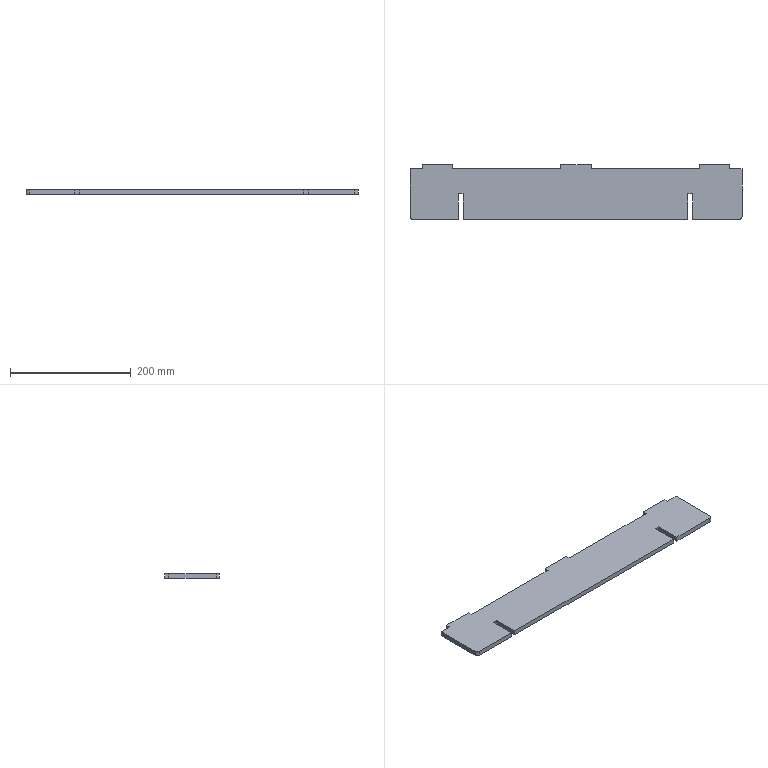Part | SolidWorks | features FlatPattern 1, SMBaseFlange 1, SheetMetal 1 | 1 solid | 28 faces | box 550 x 91 x 8 mm | volume 372474 mm3 | plane 26 | cylinder 2 | commonest cylinder face diameters 10 x2
STEP:
#1=CARTESIAN_POINT('',(176.413,-598.509,0.));
#2=VERTEX_POINT('',#1);
#3=CARTESIAN_POINT('',(156.413,-598.509,0.));
#4=VERTEX_POINT('',#3);
#5=CARTESIAN_POINT('',(176.413,-598.509,0.));
#6=DIRECTION('',(-1.,0.,0.));
#7=VECTOR('',#6,1000.);
#8=LINE('',#5,#7);
#9=EDGE_CURVE('',#2,#4,#8,.T.);
#10=ORIENTED_EDGE('',*,*,#9,.F.);
#11=CARTESIAN_POINT('',(176.413,-598.509,-8.));
#12=VERTEX_POINT('',#11);
#13=CARTESIAN_POINT('',(176.413,-598.509,-8.));
#14=DIRECTION('',(0.,0.,1.));
#15=VECTOR('',#14,1000.);
#16=LINE('',#13,#15);
#17=EDGE_CURVE('',#12,#2,#16,.T.);
#18=ORIENTED_EDGE('',*,*,#17,.F.);
#19=CARTESIAN_POINT('',(156.413,-598.509,-8.));
#20=VERTEX_POINT('',#19);
#21=CARTESIAN_POINT('',(176.413,-598.509,-8.));
#22=DIRECTION('',(-1.,0.,0.));
#23=VECTOR('',#22,1000.);
#24=LINE('',#21,#23);
#25=EDGE_CURVE('',#12,#20,#24,.T.);
#26=ORIENTED_EDGE('',*,*,#25,.T.);
#27=CARTESIAN_POINT('',(156.413,-598.509,-8.));
#28=DIRECTION('',(0.,0.,1.));
#29=VECTOR('',#28,1000.);
#30=LINE('',#27,#29);
#31=EDGE_CURVE('',#20,#4,#30,.T.);
#32=ORIENTED_EDGE('',*,*,#31,.T.);
#33=EDGE_LOOP('',(#10,#18,#26,#32));
#34=FACE_OUTER_BOUND('',#33,.T.);
#35=CARTESIAN_POINT('',(176.413,-598.509,-8.));
#36=DIRECTION('',(0.,1.,0.));
#37=DIRECTION('',(-1.,0.,0.));
#38=AXIS2_PLACEMENT_3D('',#35,#36,#37);
#39=PLANE('',#38);
#40=ADVANCED_FACE('',(#34),#39,.T.);
#41=CARTESIAN_POINT('',(176.413,-677.509,0.));
#42=VERTEX_POINT('',#41);
#43=CARTESIAN_POINT('',(176.413,-677.509,0.));
#44=DIRECTION('',(0.,1.,0.));
#45=VECTOR('',#44,1000.);
#46=LINE('',#43,#45);
#47=EDGE_CURVE('',#42,#2,#46,.T.);
#48=ORIENTED_EDGE('',*,*,#47,.F.);
#49=CARTESIAN_POINT('',(176.413,-677.509,-8.));
#50=VERTEX_POINT('',#49);
#51=CARTESIAN_POINT('',(176.413,-677.509,-8.));
#52=DIRECTION('',(0.,0.,1.));
#53=VECTOR('',#52,1000.);
#54=LINE('',#51,#53);
#55=EDGE_CURVE('',#50,#42,#54,.T.);
#56=ORIENTED_EDGE('',*,*,#55,.F.);
#57=CARTESIAN_POINT('',(176.413,-677.509,-8.));
#58=DIRECTION('',(0.,1.,0.));
#59=VECTOR('',#58,1000.);
#60=LINE('',#57,#59);
#61=EDGE_CURVE('',#50,#12,#60,.T.);
#62=ORIENTED_EDGE('',*,*,#61,.T.);
#63=ORIENTED_EDGE('',*,*,#17,.T.);
#64=EDGE_LOOP('',(#48,#56,#62,#63));
#65=FACE_OUTER_BOUND('',#64,.T.);
#66=CARTESIAN_POINT('',(176.413,-677.509,-8.));
#67=DIRECTION('',(1.,0.,0.));
#68=DIRECTION('',(0.,0.,-1.));
#69=AXIS2_PLACEMENT_3D('',#66,#67,#68);
#70=PLANE('',#69);
#71=ADVANCED_FACE('',(#65),#70,.T.);
#72=CARTESIAN_POINT('',(171.413,-682.509,0.));
#73=VERTEX_POINT('',#72);
#74=CARTESIAN_POINT('',(171.413,-677.509,0.));
#75=DIRECTION('',(0.,0.,1.));
#76=DIRECTION('',(-1.,0.,0.));
#77=AXIS2_PLACEMENT_3D('',#74,#75,#76);
#78=CIRCLE('',#77,5.);
#79=EDGE_CURVE('',#73,#42,#78,.T.);
#80=ORIENTED_EDGE('',*,*,#79,.F.);
#81=CARTESIAN_POINT('',(171.413,-682.509,-8.));
#82=VERTEX_POINT('',#81);
#83=CARTESIAN_POINT('',(171.413,-682.509,-8.));
#84=DIRECTION('',(0.,0.,1.));
#85=VECTOR('',#84,1000.);
#86=LINE('',#83,#85);
#87=EDGE_CURVE('',#82,#73,#86,.T.);
#88=ORIENTED_EDGE('',*,*,#87,.F.);
#89=CARTESIAN_POINT('',(171.413,-677.509,-8.));
#90=DIRECTION('',(0.,0.,1.));
#91=DIRECTION('',(-1.,0.,0.));
#92=AXIS2_PLACEMENT_3D('',#89,#90,#91);
#93=CIRCLE('',#92,5.);
#94=EDGE_CURVE('',#82,#50,#93,.T.);
#95=ORIENTED_EDGE('',*,*,#94,.T.);
#96=ORIENTED_EDGE('',*,*,#55,.T.);
#97=EDGE_LOOP('',(#80,#88,#95,#96));
#98=FACE_OUTER_BOUND('',#97,.T.);
#99=CARTESIAN_POINT('',(171.413,-677.509,-8.));
#100=DIRECTION('',(0.,0.,1.));
#101=DIRECTION('',(1.,0.,0.));
#102=AXIS2_PLACEMENT_3D('',#99,#100,#101);
#103=CYLINDRICAL_SURFACE('',#102,5.);
#104=ADVANCED_FACE('',(#98),#103,.T.);
#105=CARTESIAN_POINT('',(94.413,-682.509,0.));
#106=VERTEX_POINT('',#105);
#107=CARTESIAN_POINT('',(94.413,-682.509,0.));
#108=DIRECTION('',(1.,0.,0.));
#109=VECTOR('',#108,1000.);
#110=LINE('',#107,#109);
#111=EDGE_CURVE('',#106,#73,#110,.T.);
#112=ORIENTED_EDGE('',*,*,#111,.F.);
#113=CARTESIAN_POINT('',(94.413,-682.509,-8.));
#114=VERTEX_POINT('',#113);
#115=CARTESIAN_POINT('',(94.413,-682.509,-8.));
#116=DIRECTION('',(0.,0.,1.));
#117=VECTOR('',#116,1000.);
#118=LINE('',#115,#117);
#119=EDGE_CURVE('',#114,#106,#118,.T.);
#120=ORIENTED_EDGE('',*,*,#119,.F.);
#121=CARTESIAN_POINT('',(94.413,-682.509,-8.));
#122=DIRECTION('',(1.,0.,0.));
#123=VECTOR('',#122,1000.);
#124=LINE('',#121,#123);
#125=EDGE_CURVE('',#114,#82,#124,.T.);
#126=ORIENTED_EDGE('',*,*,#125,.T.);
#127=ORIENTED_EDGE('',*,*,#87,.T.);
#128=EDGE_LOOP('',(#112,#120,#126,#127));
#129=FACE_OUTER_BOUND('',#128,.T.);
#130=CARTESIAN_POINT('',(94.413,-682.509,-8.));
#131=DIRECTION('',(0.,-1.,0.));
#132=DIRECTION('',(1.,0.,0.));
#133=AXIS2_PLACEMENT_3D('',#130,#131,#132);
#134=PLANE('',#133);
#135=ADVANCED_FACE('',(#129),#134,.T.);
#136=CARTESIAN_POINT('',(94.413,-640.009,0.));
#137=VERTEX_POINT('',#136);
#138=CARTESIAN_POINT('',(94.413,-682.509,0.));
#139=DIRECTION('',(0.,-1.,0.));
#140=VECTOR('',#139,1000.);
#141=LINE('',#138,#140);
#142=EDGE_CURVE('',#137,#106,#141,.T.);
#143=ORIENTED_EDGE('',*,*,#142,.F.);
#144=CARTESIAN_POINT('',(94.413,-640.009,-8.));
#145=VERTEX_POINT('',#144);
#146=CARTESIAN_POINT('',(94.413,-640.009,-8.));
#147=DIRECTION('',(0.,0.,1.));
#148=VECTOR('',#147,1000.);
#149=LINE('',#146,#148);
#150=EDGE_CURVE('',#145,#137,#149,.T.);
#151=ORIENTED_EDGE('',*,*,#150,.F.);
#152=CARTESIAN_POINT('',(94.413,-682.509,-8.));
#153=DIRECTION('',(0.,-1.,0.));
#154=VECTOR('',#153,1000.);
#155=LINE('',#152,#154);
#156=EDGE_CURVE('',#145,#114,#155,.T.);
#157=ORIENTED_EDGE('',*,*,#156,.T.);
#158=ORIENTED_EDGE('',*,*,#119,.T.);
#159=EDGE_LOOP('',(#143,#151,#157,#158));
#160=FACE_OUTER_BOUND('',#159,.T.);
#161=CARTESIAN_POINT('',(94.413,-682.509,-8.));
#162=DIRECTION('',(-1.,0.,0.));
#163=DIRECTION('',(0.,-1.,0.));
#164=AXIS2_PLACEMENT_3D('',#161,#162,#163);
#165=PLANE('',#164);
#166=ADVANCED_FACE('',(#160),#165,.T.);
#167=CARTESIAN_POINT('',(86.413,-640.009,0.));
#168=VERTEX_POINT('',#167);
#169=CARTESIAN_POINT('',(94.413,-640.009,0.));
#170=DIRECTION('',(1.,0.,0.));
#171=VECTOR('',#170,1000.);
#172=LINE('',#169,#171);
#173=EDGE_CURVE('',#168,#137,#172,.T.);
#174=ORIENTED_EDGE('',*,*,#173,.F.);
#175=CARTESIAN_POINT('',(86.413,-640.009,-8.));
#176=VERTEX_POINT('',#175);
#177=CARTESIAN_POINT('',(86.413,-640.009,-8.));
#178=DIRECTION('',(0.,0.,1.));
#179=VECTOR('',#178,1000.);
#180=LINE('',#177,#179);
#181=EDGE_CURVE('',#176,#168,#180,.T.);
#182=ORIENTED_EDGE('',*,*,#181,.F.);
#183=CARTESIAN_POINT('',(94.413,-640.009,-8.));
#184=DIRECTION('',(1.,0.,0.));
#185=VECTOR('',#184,1000.);
#186=LINE('',#183,#185);
#187=EDGE_CURVE('',#176,#145,#186,.T.);
#188=ORIENTED_EDGE('',*,*,#187,.T.);
#189=ORIENTED_EDGE('',*,*,#150,.T.);
#190=EDGE_LOOP('',(#174,#182,#188,#189));
#191=FACE_OUTER_BOUND('',#190,.T.);
#192=CARTESIAN_POINT('',(94.413,-640.009,-8.));
#193=DIRECTION('',(0.,-1.,0.));
#194=DIRECTION('',(0.,0.,-1.));
#195=AXIS2_PLACEMENT_3D('',#192,#193,#194);
#196=PLANE('',#195);
#197=ADVANCED_FACE('',(#191),#196,.T.);
#198=CARTESIAN_POINT('',(86.413,-682.509,0.));
#199=VERTEX_POINT('',#198);
#200=CARTESIAN_POINT('',(86.413,-640.009,0.));
#201=DIRECTION('',(0.,1.,0.));
#202=VECTOR('',#201,1000.);
#203=LINE('',#200,#202);
#204=EDGE_CURVE('',#199,#168,#203,.T.);
#205=ORIENTED_EDGE('',*,*,#204,.F.);
#206=CARTESIAN_POINT('',(86.413,-682.509,-8.));
#207=VERTEX_POINT('',#206);
#208=CARTESIAN_POINT('',(86.413,-682.509,-8.));
#209=DIRECTION('',(0.,0.,1.));
#210=VECTOR('',#209,1000.);
#211=LINE('',#208,#210);
#212=EDGE_CURVE('',#207,#199,#211,.T.);
#213=ORIENTED_EDGE('',*,*,#212,.F.);
#214=CARTESIAN_POINT('',(86.413,-640.009,-8.));
#215=DIRECTION('',(0.,1.,0.));
#216=VECTOR('',#215,1000.);
#217=LINE('',#214,#216);
#218=EDGE_CURVE('',#207,#176,#217,.T.);
#219=ORIENTED_EDGE('',*,*,#218,.T.);
#220=ORIENTED_EDGE('',*,*,#181,.T.);
#221=EDGE_LOOP('',(#205,#213,#219,#220));
#222=FACE_OUTER_BOUND('',#221,.T.);
#223=CARTESIAN_POINT('',(86.413,-640.009,-8.));
#224=DIRECTION('',(1.,0.,0.));
#225=DIRECTION('',(0.,1.,0.));
#226=AXIS2_PLACEMENT_3D('',#223,#224,#225);
#227=PLANE('',#226);
#228=ADVANCED_FACE('',(#222),#227,.T.);
#229=CARTESIAN_POINT('',(-285.587,-682.509,0.));
#230=VERTEX_POINT('',#229);
#231=CARTESIAN_POINT('',(-285.587,-682.509,0.));
#232=DIRECTION('',(1.,0.,0.));
#233=VECTOR('',#232,1000.);
#234=LINE('',#231,#233);
#235=EDGE_CURVE('',#230,#199,#234,.T.);
#236=ORIENTED_EDGE('',*,*,#235,.F.);
#237=CARTESIAN_POINT('',(-285.587,-682.509,-8.));
#238=VERTEX_POINT('',#237);
#239=CARTESIAN_POINT('',(-285.587,-682.509,-8.));
#240=DIRECTION('',(0.,0.,1.));
#241=VECTOR('',#240,1000.);
#242=LINE('',#239,#241);
#243=EDGE_CURVE('',#238,#230,#242,.T.);
#244=ORIENTED_EDGE('',*,*,#243,.F.);
#245=CARTESIAN_POINT('',(-285.587,-682.509,-8.));
#246=DIRECTION('',(1.,0.,0.));
#247=VECTOR('',#246,1000.);
#248=LINE('',#245,#247);
#249=EDGE_CURVE('',#238,#207,#248,.T.);
#250=ORIENTED_EDGE('',*,*,#249,.T.);
#251=ORIENTED_EDGE('',*,*,#212,.T.);
#252=EDGE_LOOP('',(#236,#244,#250,#251));
#253=FACE_OUTER_BOUND('',#252,.T.);
#254=CARTESIAN_POINT('',(-285.587,-682.509,-8.));
#255=DIRECTION('',(0.,-1.,0.));
#256=DIRECTION('',(1.,0.,0.));
#257=AXIS2_PLACEMENT_3D('',#254,#255,#256);
#258=PLANE('',#257);
#259=ADVANCED_FACE('',(#253),#258,.T.);
#260=CARTESIAN_POINT('',(-285.587,-640.009,0.));
#261=VERTEX_POINT('',#260);
#262=CARTESIAN_POINT('',(-285.587,-682.509,0.));
#263=DIRECTION('',(0.,-1.,0.));
#264=VECTOR('',#263,1000.);
#265=LINE('',#262,#264);
#266=EDGE_CURVE('',#261,#230,#265,.T.);
#267=ORIENTED_EDGE('',*,*,#266,.F.);
#268=CARTESIAN_POINT('',(-285.587,-640.009,-8.));
#269=VERTEX_POINT('',#268);
#270=CARTESIAN_POINT('',(-285.587,-640.009,-8.));
#271=DIRECTION('',(0.,0.,1.));
#272=VECTOR('',#271,1000.);
#273=LINE('',#270,#272);
#274=EDGE_CURVE('',#269,#261,#273,.T.);
#275=ORIENTED_EDGE('',*,*,#274,.F.);
#276=CARTESIAN_POINT('',(-285.587,-682.509,-8.));
#277=DIRECTION('',(0.,-1.,0.));
#278=VECTOR('',#277,1000.);
#279=LINE('',#276,#278);
#280=EDGE_CURVE('',#269,#238,#279,.T.);
#281=ORIENTED_EDGE('',*,*,#280,.T.);
#282=ORIENTED_EDGE('',*,*,#243,.T.);
#283=EDGE_LOOP('',(#267,#275,#281,#282));
#284=FACE_OUTER_BOUND('',#283,.T.);
#285=CARTESIAN_POINT('',(-285.587,-682.509,-8.));
#286=DIRECTION('',(-1.,0.,0.));
#287=DIRECTION('',(0.,-1.,0.));
#288=AXIS2_PLACEMENT_3D('',#285,#286,#287);
#289=PLANE('',#288);
#290=ADVANCED_FACE('',(#284),#289,.T.);
#291=CARTESIAN_POINT('',(-293.587,-640.009,0.));
#292=VERTEX_POINT('',#291);
#293=CARTESIAN_POINT('',(-285.587,-640.009,0.));
#294=DIRECTION('',(1.,0.,0.));
#295=VECTOR('',#294,1000.);
#296=LINE('',#293,#295);
#297=EDGE_CURVE('',#292,#261,#296,.T.);
#298=ORIENTED_EDGE('',*,*,#297,.F.);
#299=CARTESIAN_POINT('',(-293.587,-640.009,-8.));
#300=VERTEX_POINT('',#299);
#301=CARTESIAN_POINT('',(-293.587,-640.009,-8.));
#302=DIRECTION('',(0.,0.,1.));
#303=VECTOR('',#302,1000.);
#304=LINE('',#301,#303);
#305=EDGE_CURVE('',#300,#292,#304,.T.);
#306=ORIENTED_EDGE('',*,*,#305,.F.);
#307=CARTESIAN_POINT('',(-285.587,-640.009,-8.));
#308=DIRECTION('',(1.,0.,0.));
#309=VECTOR('',#308,1000.);
#310=LINE('',#307,#309);
#311=EDGE_CURVE('',#300,#269,#310,.T.);
#312=ORIENTED_EDGE('',*,*,#311,.T.);
#313=ORIENTED_EDGE('',*,*,#274,.T.);
#314=EDGE_LOOP('',(#298,#306,#312,#313));
#315=FACE_OUTER_BOUND('',#314,.T.);
#316=CARTESIAN_POINT('',(-285.587,-640.009,-8.));
#317=DIRECTION('',(0.,-1.,0.));
#318=DIRECTION('',(0.,0.,-1.));
#319=AXIS2_PLACEMENT_3D('',#316,#317,#318);
#320=PLANE('',#319);
#321=ADVANCED_FACE('',(#315),#320,.T.);
#322=CARTESIAN_POINT('',(-293.587,-682.509,0.));
#323=VERTEX_POINT('',#322);
#324=CARTESIAN_POINT('',(-293.587,-640.009,0.));
#325=DIRECTION('',(0.,1.,0.));
#326=VECTOR('',#325,1000.);
#327=LINE('',#324,#326);
#328=EDGE_CURVE('',#323,#292,#327,.T.);
#329=ORIENTED_EDGE('',*,*,#328,.F.);
#330=CARTESIAN_POINT('',(-293.587,-682.509,-8.));
#331=VERTEX_POINT('',#330);
#332=CARTESIAN_POINT('',(-293.587,-682.509,-8.));
#333=DIRECTION('',(0.,0.,1.));
#334=VECTOR('',#333,1000.);
#335=LINE('',#332,#334);
#336=EDGE_CURVE('',#331,#323,#335,.T.);
#337=ORIENTED_EDGE('',*,*,#336,.F.);
#338=CARTESIAN_POINT('',(-293.587,-640.009,-8.));
#339=DIRECTION('',(0.,1.,0.));
#340=VECTOR('',#339,1000.);
#341=LINE('',#338,#340);
#342=EDGE_CURVE('',#331,#300,#341,.T.);
#343=ORIENTED_EDGE('',*,*,#342,.T.);
#344=ORIENTED_EDGE('',*,*,#305,.T.);
#345=EDGE_LOOP('',(#329,#337,#343,#344));
#346=FACE_OUTER_BOUND('',#345,.T.);
#347=CARTESIAN_POINT('',(-293.587,-640.009,-8.));
#348=DIRECTION('',(1.,0.,0.));
#349=DIRECTION('',(0.,1.,0.));
#350=AXIS2_PLACEMENT_3D('',#347,#348,#349);
#351=PLANE('',#350);
#352=ADVANCED_FACE('',(#346),#351,.T.);
#353=CARTESIAN_POINT('',(-368.587,-682.509,0.));
#354=VERTEX_POINT('',#353);
#355=CARTESIAN_POINT('',(-368.587,-682.509,0.));
#356=DIRECTION('',(1.,0.,0.));
#357=VECTOR('',#356,1000.);
#358=LINE('',#355,#357);
#359=EDGE_CURVE('',#354,#323,#358,.T.);
#360=ORIENTED_EDGE('',*,*,#359,.F.);
#361=CARTESIAN_POINT('',(-368.587,-682.509,-8.));
#362=VERTEX_POINT('',#361);
#363=CARTESIAN_POINT('',(-368.587,-682.509,-8.));
#364=DIRECTION('',(0.,0.,1.));
#365=VECTOR('',#364,1000.);
#366=LINE('',#363,#365);
#367=EDGE_CURVE('',#362,#354,#366,.T.);
#368=ORIENTED_EDGE('',*,*,#367,.F.);
#369=CARTESIAN_POINT('',(-368.587,-682.509,-8.));
#370=DIRECTION('',(1.,0.,0.));
#371=VECTOR('',#370,1000.);
#372=LINE('',#369,#371);
#373=EDGE_CURVE('',#362,#331,#372,.T.);
#374=ORIENTED_EDGE('',*,*,#373,.T.);
#375=ORIENTED_EDGE('',*,*,#336,.T.);
#376=EDGE_LOOP('',(#360,#368,#374,#375));
#377=FACE_OUTER_BOUND('',#376,.T.);
#378=CARTESIAN_POINT('',(-368.587,-682.509,-8.));
#379=DIRECTION('',(0.,-1.,0.));
#380=DIRECTION('',(1.,0.,0.));
#381=AXIS2_PLACEMENT_3D('',#378,#379,#380);
#382=PLANE('',#381);
#383=ADVANCED_FACE('',(#377),#382,.T.);
#384=CARTESIAN_POINT('',(-373.587,-677.509,0.));
#385=VERTEX_POINT('',#384);
#386=CARTESIAN_POINT('',(-368.587,-677.509,0.));
#387=DIRECTION('',(0.,0.,1.));
#388=DIRECTION('',(1.,0.,0.));
#389=AXIS2_PLACEMENT_3D('',#386,#387,#388);
#390=CIRCLE('',#389,5.);
#391=EDGE_CURVE('',#385,#354,#390,.T.);
#392=ORIENTED_EDGE('',*,*,#391,.F.);
#393=CARTESIAN_POINT('',(-373.587,-677.509,-8.));
#394=VERTEX_POINT('',#393);
#395=CARTESIAN_POINT('',(-373.587,-677.509,-8.));
#396=DIRECTION('',(0.,0.,1.));
#397=VECTOR('',#396,1000.);
#398=LINE('',#395,#397);
#399=EDGE_CURVE('',#394,#385,#398,.T.);
#400=ORIENTED_EDGE('',*,*,#399,.F.);
#401=CARTESIAN_POINT('',(-368.587,-677.509,-8.));
#402=DIRECTION('',(0.,0.,1.));
#403=DIRECTION('',(1.,0.,0.));
#404=AXIS2_PLACEMENT_3D('',#401,#402,#403);
#405=CIRCLE('',#404,5.);
#406=EDGE_CURVE('',#394,#362,#405,.T.);
#407=ORIENTED_EDGE('',*,*,#406,.T.);
#408=ORIENTED_EDGE('',*,*,#367,.T.);
#409=EDGE_LOOP('',(#392,#400,#407,#408));
#410=FACE_OUTER_BOUND('',#409,.T.);
#411=CARTESIAN_POINT('',(-368.587,-677.509,-8.));
#412=DIRECTION('',(0.,0.,1.));
#413=DIRECTION('',(1.,0.,0.));
#414=AXIS2_PLACEMENT_3D('',#411,#412,#413);
#415=CYLINDRICAL_SURFACE('',#414,5.);
#416=ADVANCED_FACE('',(#410),#415,.T.);
#417=CARTESIAN_POINT('',(-373.587,-598.509,0.));
#418=VERTEX_POINT('',#417);
#419=CARTESIAN_POINT('',(-373.587,-598.509,0.));
#420=DIRECTION('',(0.,-1.,0.));
#421=VECTOR('',#420,1000.);
#422=LINE('',#419,#421);
#423=EDGE_CURVE('',#418,#385,#422,.T.);
#424=ORIENTED_EDGE('',*,*,#423,.F.);
#425=CARTESIAN_POINT('',(-373.587,-598.509,-8.));
#426=VERTEX_POINT('',#425);
#427=CARTESIAN_POINT('',(-373.587,-598.509,-8.));
#428=DIRECTION('',(0.,0.,1.));
#429=VECTOR('',#428,1000.);
#430=LINE('',#427,#429);
#431=EDGE_CURVE('',#426,#418,#430,.T.);
#432=ORIENTED_EDGE('',*,*,#431,.F.);
#433=CARTESIAN_POINT('',(-373.587,-598.509,-8.));
#434=DIRECTION('',(0.,-1.,0.));
#435=VECTOR('',#434,1000.);
#436=LINE('',#433,#435);
#437=EDGE_CURVE('',#426,#394,#436,.T.);
#438=ORIENTED_EDGE('',*,*,#437,.T.);
#439=ORIENTED_EDGE('',*,*,#399,.T.);
#440=EDGE_LOOP('',(#424,#432,#438,#439));
#441=FACE_OUTER_BOUND('',#440,.T.);
#442=CARTESIAN_POINT('',(-373.587,-598.509,-8.));
#443=DIRECTION('',(-1.,0.,0.));
#444=DIRECTION('',(0.,-1.,0.));
#445=AXIS2_PLACEMENT_3D('',#442,#443,#444);
#446=PLANE('',#445);
#447=ADVANCED_FACE('',(#441),#446,.T.);
#448=CARTESIAN_POINT('',(-353.587,-598.509,0.));
#449=VERTEX_POINT('',#448);
#450=CARTESIAN_POINT('',(-353.587,-598.509,0.));
#451=DIRECTION('',(-1.,0.,0.));
#452=VECTOR('',#451,1000.);
#453=LINE('',#450,#452);
#454=EDGE_CURVE('',#449,#418,#453,.T.);
#455=ORIENTED_EDGE('',*,*,#454,.F.);
#456=CARTESIAN_POINT('',(-353.587,-598.509,-8.));
#457=VERTEX_POINT('',#456);
#458=CARTESIAN_POINT('',(-353.587,-598.509,-8.));
#459=DIRECTION('',(0.,0.,1.));
#460=VECTOR('',#459,1000.);
#461=LINE('',#458,#460);
#462=EDGE_CURVE('',#457,#449,#461,.T.);
#463=ORIENTED_EDGE('',*,*,#462,.F.);
#464=CARTESIAN_POINT('',(-353.587,-598.509,-8.));
#465=DIRECTION('',(-1.,0.,0.));
#466=VECTOR('',#465,1000.);
#467=LINE('',#464,#466);
#468=EDGE_CURVE('',#457,#426,#467,.T.);
#469=ORIENTED_EDGE('',*,*,#468,.T.);
#470=ORIENTED_EDGE('',*,*,#431,.T.);
#471=EDGE_LOOP('',(#455,#463,#469,#470));
#472=FACE_OUTER_BOUND('',#471,.T.);
#473=CARTESIAN_POINT('',(-353.587,-598.509,-8.));
#474=DIRECTION('',(0.,1.,0.));
#475=DIRECTION('',(0.,0.,1.));
#476=AXIS2_PLACEMENT_3D('',#473,#474,#475);
#477=PLANE('',#476);
#478=ADVANCED_FACE('',(#472),#477,.T.);
#479=CARTESIAN_POINT('',(-353.587,-591.509,0.));
#480=VERTEX_POINT('',#479);
#481=CARTESIAN_POINT('',(-353.587,-591.509,0.));
#482=DIRECTION('',(0.,-1.,0.));
#483=VECTOR('',#482,1000.);
#484=LINE('',#481,#483);
#485=EDGE_CURVE('',#480,#449,#484,.T.);
#486=ORIENTED_EDGE('',*,*,#485,.F.);
#487=CARTESIAN_POINT('',(-353.587,-591.509,-8.));
#488=VERTEX_POINT('',#487);
#489=CARTESIAN_POINT('',(-353.587,-591.509,-8.));
#490=DIRECTION('',(0.,0.,1.));
#491=VECTOR('',#490,1000.);
#492=LINE('',#489,#491);
#493=EDGE_CURVE('',#488,#480,#492,.T.);
#494=ORIENTED_EDGE('',*,*,#493,.F.);
#495=CARTESIAN_POINT('',(-353.587,-591.509,-8.));
#496=DIRECTION('',(0.,-1.,0.));
#497=VECTOR('',#496,1000.);
#498=LINE('',#495,#497);
#499=EDGE_CURVE('',#488,#457,#498,.T.);
#500=ORIENTED_EDGE('',*,*,#499,.T.);
#501=ORIENTED_EDGE('',*,*,#462,.T.);
#502=EDGE_LOOP('',(#486,#494,#500,#501));
#503=FACE_OUTER_BOUND('',#502,.T.);
#504=CARTESIAN_POINT('',(-353.587,-591.509,-8.));
#505=DIRECTION('',(-1.,0.,0.));
#506=DIRECTION('',(0.,0.,1.));
#507=AXIS2_PLACEMENT_3D('',#504,#505,#506);
#508=PLANE('',#507);
#509=ADVANCED_FACE('',(#503),#508,.T.);
#510=CARTESIAN_POINT('',(-303.587,-591.509,0.));
#511=VERTEX_POINT('',#510);
#512=CARTESIAN_POINT('',(-303.587,-591.509,0.));
#513=DIRECTION('',(-1.,0.,0.));
#514=VECTOR('',#513,1000.);
#515=LINE('',#512,#514);
#516=EDGE_CURVE('',#511,#480,#515,.T.);
#517=ORIENTED_EDGE('',*,*,#516,.F.);
#518=CARTESIAN_POINT('',(-303.587,-591.509,-8.));
#519=VERTEX_POINT('',#518);
#520=CARTESIAN_POINT('',(-303.587,-591.509,-8.));
#521=DIRECTION('',(0.,0.,1.));
#522=VECTOR('',#521,1000.);
#523=LINE('',#520,#522);
#524=EDGE_CURVE('',#519,#511,#523,.T.);
#525=ORIENTED_EDGE('',*,*,#524,.F.);
#526=CARTESIAN_POINT('',(-303.587,-591.509,-8.));
#527=DIRECTION('',(-1.,0.,0.));
#528=VECTOR('',#527,1000.);
#529=LINE('',#526,#528);
#530=EDGE_CURVE('',#519,#488,#529,.T.);
#531=ORIENTED_EDGE('',*,*,#530,.T.);
#532=ORIENTED_EDGE('',*,*,#493,.T.);
#533=EDGE_LOOP('',(#517,#525,#531,#532));
#534=FACE_OUTER_BOUND('',#533,.T.);
#535=CARTESIAN_POINT('',(-303.587,-591.509,-8.));
#536=DIRECTION('',(0.,1.,0.));
#537=DIRECTION('',(0.,0.,1.));
#538=AXIS2_PLACEMENT_3D('',#535,#536,#537);
#539=PLANE('',#538);
#540=ADVANCED_FACE('',(#534),#539,.T.);
#541=CARTESIAN_POINT('',(-303.587,-598.509,0.));
#542=VERTEX_POINT('',#541);
#543=CARTESIAN_POINT('',(-303.587,-598.509,0.));
#544=DIRECTION('',(0.,1.,0.));
#545=VECTOR('',#544,1000.);
#546=LINE('',#543,#545);
#547=EDGE_CURVE('',#542,#511,#546,.T.);
#548=ORIENTED_EDGE('',*,*,#547,.F.);
#549=CARTESIAN_POINT('',(-303.587,-598.509,-8.));
#550=VERTEX_POINT('',#549);
#551=CARTESIAN_POINT('',(-303.587,-598.509,-8.));
#552=DIRECTION('',(0.,0.,1.));
#553=VECTOR('',#552,1000.);
#554=LINE('',#551,#553);
#555=EDGE_CURVE('',#550,#542,#554,.T.);
#556=ORIENTED_EDGE('',*,*,#555,.F.);
#557=CARTESIAN_POINT('',(-303.587,-598.509,-8.));
#558=DIRECTION('',(0.,1.,0.));
#559=VECTOR('',#558,1000.);
#560=LINE('',#557,#559);
#561=EDGE_CURVE('',#550,#519,#560,.T.);
#562=ORIENTED_EDGE('',*,*,#561,.T.);
#563=ORIENTED_EDGE('',*,*,#524,.T.);
#564=EDGE_LOOP('',(#548,#556,#562,#563));
#565=FACE_OUTER_BOUND('',#564,.T.);
#566=CARTESIAN_POINT('',(-303.587,-598.509,-8.));
#567=DIRECTION('',(1.,0.,0.));
#568=DIRECTION('',(0.,0.,-1.));
#569=AXIS2_PLACEMENT_3D('',#566,#567,#568);
#570=PLANE('',#569);
#571=ADVANCED_FACE('',(#565),#570,.T.);
#572=CARTESIAN_POINT('',(-123.587,-598.509,0.));
#573=VERTEX_POINT('',#572);
#574=CARTESIAN_POINT('',(-123.587,-598.509,0.));
#575=DIRECTION('',(-1.,0.,0.));
#576=VECTOR('',#575,1000.);
#577=LINE('',#574,#576);
#578=EDGE_CURVE('',#573,#542,#577,.T.);
#579=ORIENTED_EDGE('',*,*,#578,.F.);
#580=CARTESIAN_POINT('',(-123.587,-598.509,-8.));
#581=VERTEX_POINT('',#580);
#582=CARTESIAN_POINT('',(-123.587,-598.509,-8.));
#583=DIRECTION('',(0.,0.,1.));
#584=VECTOR('',#583,1000.);
#585=LINE('',#582,#584);
#586=EDGE_CURVE('',#581,#573,#585,.T.);
#587=ORIENTED_EDGE('',*,*,#586,.F.);
#588=CARTESIAN_POINT('',(-123.587,-598.509,-8.));
#589=DIRECTION('',(-1.,0.,0.));
#590=VECTOR('',#589,1000.);
#591=LINE('',#588,#590);
#592=EDGE_CURVE('',#581,#550,#591,.T.);
#593=ORIENTED_EDGE('',*,*,#592,.T.);
#594=ORIENTED_EDGE('',*,*,#555,.T.);
#595=EDGE_LOOP('',(#579,#587,#593,#594));
#596=FACE_OUTER_BOUND('',#595,.T.);
#597=CARTESIAN_POINT('',(-123.587,-598.509,-8.));
#598=DIRECTION('',(0.,1.,0.));
#599=DIRECTION('',(-1.,0.,0.));
#600=AXIS2_PLACEMENT_3D('',#597,#598,#599);
#601=PLANE('',#600);
#602=ADVANCED_FACE('',(#596),#601,.T.);
#603=CARTESIAN_POINT('',(-123.587,-591.509,0.));
#604=VERTEX_POINT('',#603);
#605=CARTESIAN_POINT('',(-123.587,-591.509,0.));
#606=DIRECTION('',(0.,-1.,0.));
#607=VECTOR('',#606,1000.);
#608=LINE('',#605,#607);
#609=EDGE_CURVE('',#604,#573,#608,.T.);
#610=ORIENTED_EDGE('',*,*,#609,.F.);
#611=CARTESIAN_POINT('',(-123.587,-591.509,-8.));
#612=VERTEX_POINT('',#611);
#613=CARTESIAN_POINT('',(-123.587,-591.509,-8.));
#614=DIRECTION('',(0.,0.,1.));
#615=VECTOR('',#614,1000.);
#616=LINE('',#613,#615);
#617=EDGE_CURVE('',#612,#604,#616,.T.);
#618=ORIENTED_EDGE('',*,*,#617,.F.);
#619=CARTESIAN_POINT('',(-123.587,-591.509,-8.));
#620=DIRECTION('',(0.,-1.,0.));
#621=VECTOR('',#620,1000.);
#622=LINE('',#619,#621);
#623=EDGE_CURVE('',#612,#581,#622,.T.);
#624=ORIENTED_EDGE('',*,*,#623,.T.);
#625=ORIENTED_EDGE('',*,*,#586,.T.);
#626=EDGE_LOOP('',(#610,#618,#624,#625));
#627=FACE_OUTER_BOUND('',#626,.T.);
#628=CARTESIAN_POINT('',(-123.587,-591.509,-8.));
#629=DIRECTION('',(-1.,0.,0.));
#630=DIRECTION('',(0.,0.,1.));
#631=AXIS2_PLACEMENT_3D('',#628,#629,#630);
#632=PLANE('',#631);
#633=ADVANCED_FACE('',(#627),#632,.T.);
#634=CARTESIAN_POINT('',(-73.587,-591.509,0.));
#635=VERTEX_POINT('',#634);
#636=CARTESIAN_POINT('',(-73.587,-591.509,0.));
#637=DIRECTION('',(-1.,0.,0.));
#638=VECTOR('',#637,1000.);
#639=LINE('',#636,#638);
#640=EDGE_CURVE('',#635,#604,#639,.T.);
#641=ORIENTED_EDGE('',*,*,#640,.F.);
#642=CARTESIAN_POINT('',(-73.587,-591.509,-8.));
#643=VERTEX_POINT('',#642);
#644=CARTESIAN_POINT('',(-73.587,-591.509,-8.));
#645=DIRECTION('',(0.,0.,1.));
#646=VECTOR('',#645,1000.);
#647=LINE('',#644,#646);
#648=EDGE_CURVE('',#643,#635,#647,.T.);
#649=ORIENTED_EDGE('',*,*,#648,.F.);
#650=CARTESIAN_POINT('',(-73.587,-591.509,-8.));
#651=DIRECTION('',(-1.,0.,0.));
#652=VECTOR('',#651,1000.);
#653=LINE('',#650,#652);
#654=EDGE_CURVE('',#643,#612,#653,.T.);
#655=ORIENTED_EDGE('',*,*,#654,.T.);
#656=ORIENTED_EDGE('',*,*,#617,.T.);
#657=EDGE_LOOP('',(#641,#649,#655,#656));
#658=FACE_OUTER_BOUND('',#657,.T.);
#659=CARTESIAN_POINT('',(-73.587,-591.509,-8.));
#660=DIRECTION('',(0.,1.,0.));
#661=DIRECTION('',(0.,0.,1.));
#662=AXIS2_PLACEMENT_3D('',#659,#660,#661);
#663=PLANE('',#662);
#664=ADVANCED_FACE('',(#658),#663,.T.);
#665=CARTESIAN_POINT('',(-73.587,-598.509,0.));
#666=VERTEX_POINT('',#665);
#667=CARTESIAN_POINT('',(-73.587,-598.509,0.));
#668=DIRECTION('',(0.,1.,0.));
#669=VECTOR('',#668,1000.);
#670=LINE('',#667,#669);
#671=EDGE_CURVE('',#666,#635,#670,.T.);
#672=ORIENTED_EDGE('',*,*,#671,.F.);
#673=CARTESIAN_POINT('',(-73.587,-598.509,-8.));
#674=VERTEX_POINT('',#673);
#675=CARTESIAN_POINT('',(-73.587,-598.509,-8.));
#676=DIRECTION('',(0.,0.,1.));
#677=VECTOR('',#676,1000.);
#678=LINE('',#675,#677);
#679=EDGE_CURVE('',#674,#666,#678,.T.);
#680=ORIENTED_EDGE('',*,*,#679,.F.);
#681=CARTESIAN_POINT('',(-73.587,-598.509,-8.));
#682=DIRECTION('',(0.,1.,0.));
#683=VECTOR('',#682,1000.);
#684=LINE('',#681,#683);
#685=EDGE_CURVE('',#674,#643,#684,.T.);
#686=ORIENTED_EDGE('',*,*,#685,.T.);
#687=ORIENTED_EDGE('',*,*,#648,.T.);
#688=EDGE_LOOP('',(#672,#680,#686,#687));
#689=FACE_OUTER_BOUND('',#688,.T.);
#690=CARTESIAN_POINT('',(-73.587,-598.509,-8.));
#691=DIRECTION('',(1.,0.,0.));
#692=DIRECTION('',(0.,0.,-1.));
#693=AXIS2_PLACEMENT_3D('',#690,#691,#692);
#694=PLANE('',#693);
#695=ADVANCED_FACE('',(#689),#694,.T.);
#696=CARTESIAN_POINT('',(106.413,-598.509,0.));
#697=VERTEX_POINT('',#696);
#698=CARTESIAN_POINT('',(106.413,-598.509,0.));
#699=DIRECTION('',(-1.,0.,0.));
#700=VECTOR('',#699,1000.);
#701=LINE('',#698,#700);
#702=EDGE_CURVE('',#697,#666,#701,.T.);
#703=ORIENTED_EDGE('',*,*,#702,.F.);
#704=CARTESIAN_POINT('',(106.413,-598.509,-8.));
#705=VERTEX_POINT('',#704);
#706=CARTESIAN_POINT('',(106.413,-598.509,-8.));
#707=DIRECTION('',(0.,0.,1.));
#708=VECTOR('',#707,1000.);
#709=LINE('',#706,#708);
#710=EDGE_CURVE('',#705,#697,#709,.T.);
#711=ORIENTED_EDGE('',*,*,#710,.F.);
#712=CARTESIAN_POINT('',(106.413,-598.509,-8.));
#713=DIRECTION('',(-1.,0.,0.));
#714=VECTOR('',#713,1000.);
#715=LINE('',#712,#714);
#716=EDGE_CURVE('',#705,#674,#715,.T.);
#717=ORIENTED_EDGE('',*,*,#716,.T.);
#718=ORIENTED_EDGE('',*,*,#679,.T.);
#719=EDGE_LOOP('',(#703,#711,#717,#718));
#720=FACE_OUTER_BOUND('',#719,.T.);
#721=CARTESIAN_POINT('',(106.413,-598.509,-8.));
#722=DIRECTION('',(0.,1.,0.));
#723=DIRECTION('',(0.,0.,1.));
#724=AXIS2_PLACEMENT_3D('',#721,#722,#723);
#725=PLANE('',#724);
#726=ADVANCED_FACE('',(#720),#725,.T.);
#727=CARTESIAN_POINT('',(106.413,-591.509,0.));
#728=VERTEX_POINT('',#727);
#729=CARTESIAN_POINT('',(106.413,-591.509,0.));
#730=DIRECTION('',(0.,-1.,0.));
#731=VECTOR('',#730,1000.);
#732=LINE('',#729,#731);
#733=EDGE_CURVE('',#728,#697,#732,.T.);
#734=ORIENTED_EDGE('',*,*,#733,.F.);
#735=CARTESIAN_POINT('',(106.413,-591.509,-8.));
#736=VERTEX_POINT('',#735);
#737=CARTESIAN_POINT('',(106.413,-591.509,-8.));
#738=DIRECTION('',(0.,0.,1.));
#739=VECTOR('',#738,1000.);
#740=LINE('',#737,#739);
#741=EDGE_CURVE('',#736,#728,#740,.T.);
#742=ORIENTED_EDGE('',*,*,#741,.F.);
#743=CARTESIAN_POINT('',(106.413,-591.509,-8.));
#744=DIRECTION('',(0.,-1.,0.));
#745=VECTOR('',#744,1000.);
#746=LINE('',#743,#745);
#747=EDGE_CURVE('',#736,#705,#746,.T.);
#748=ORIENTED_EDGE('',*,*,#747,.T.);
#749=ORIENTED_EDGE('',*,*,#710,.T.);
#750=EDGE_LOOP('',(#734,#742,#748,#749));
#751=FACE_OUTER_BOUND('',#750,.T.);
#752=CARTESIAN_POINT('',(106.413,-591.509,-8.));
#753=DIRECTION('',(-1.,0.,0.));
#754=DIRECTION('',(0.,-1.,0.));
#755=AXIS2_PLACEMENT_3D('',#752,#753,#754);
#756=PLANE('',#755);
#757=ADVANCED_FACE('',(#751),#756,.T.);
#758=CARTESIAN_POINT('',(156.413,-591.509,0.));
#759=VERTEX_POINT('',#758);
#760=CARTESIAN_POINT('',(156.413,-591.509,0.));
#761=DIRECTION('',(-1.,0.,0.));
#762=VECTOR('',#761,1000.);
#763=LINE('',#760,#762);
#764=EDGE_CURVE('',#759,#728,#763,.T.);
#765=ORIENTED_EDGE('',*,*,#764,.F.);
#766=CARTESIAN_POINT('',(156.413,-591.509,-8.));
#767=VERTEX_POINT('',#766);
#768=CARTESIAN_POINT('',(156.413,-591.509,-8.));
#769=DIRECTION('',(0.,0.,1.));
#770=VECTOR('',#769,1000.);
#771=LINE('',#768,#770);
#772=EDGE_CURVE('',#767,#759,#771,.T.);
#773=ORIENTED_EDGE('',*,*,#772,.F.);
#774=CARTESIAN_POINT('',(156.413,-591.509,-8.));
#775=DIRECTION('',(-1.,0.,0.));
#776=VECTOR('',#775,1000.);
#777=LINE('',#774,#776);
#778=EDGE_CURVE('',#767,#736,#777,.T.);
#779=ORIENTED_EDGE('',*,*,#778,.T.);
#780=ORIENTED_EDGE('',*,*,#741,.T.);
#781=EDGE_LOOP('',(#765,#773,#779,#780));
#782=FACE_OUTER_BOUND('',#781,.T.);
#783=CARTESIAN_POINT('',(156.413,-591.509,-8.));
#784=DIRECTION('',(0.,1.,0.));
#785=DIRECTION('',(0.,0.,1.));
#786=AXIS2_PLACEMENT_3D('',#783,#784,#785);
#787=PLANE('',#786);
#788=ADVANCED_FACE('',(#782),#787,.T.);
#789=CARTESIAN_POINT('',(156.413,-598.509,0.));
#790=DIRECTION('',(0.,1.,0.));
#791=VECTOR('',#790,1000.);
#792=LINE('',#789,#791);
#793=EDGE_CURVE('',#4,#759,#792,.T.);
#794=ORIENTED_EDGE('',*,*,#793,.F.);
#795=ORIENTED_EDGE('',*,*,#31,.F.);
#796=CARTESIAN_POINT('',(156.413,-598.509,-8.));
#797=DIRECTION('',(0.,1.,0.));
#798=VECTOR('',#797,1000.);
#799=LINE('',#796,#798);
#800=EDGE_CURVE('',#20,#767,#799,.T.);
#801=ORIENTED_EDGE('',*,*,#800,.T.);
#802=ORIENTED_EDGE('',*,*,#772,.T.);
#803=EDGE_LOOP('',(#794,#795,#801,#802));
#804=FACE_OUTER_BOUND('',#803,.T.);
#805=CARTESIAN_POINT('',(156.413,-598.509,-8.));
#806=DIRECTION('',(1.,0.,0.));
#807=DIRECTION('',(0.,1.,0.));
#808=AXIS2_PLACEMENT_3D('',#805,#806,#807);
#809=PLANE('',#808);
#810=ADVANCED_FACE('',(#804),#809,.T.);
#811=ORIENTED_EDGE('',*,*,#25,.F.);
#812=ORIENTED_EDGE('',*,*,#61,.F.);
#813=ORIENTED_EDGE('',*,*,#94,.F.);
#814=ORIENTED_EDGE('',*,*,#125,.F.);
#815=ORIENTED_EDGE('',*,*,#156,.F.);
#816=ORIENTED_EDGE('',*,*,#187,.F.);
#817=ORIENTED_EDGE('',*,*,#218,.F.);
#818=ORIENTED_EDGE('',*,*,#249,.F.);
#819=ORIENTED_EDGE('',*,*,#280,.F.);
#820=ORIENTED_EDGE('',*,*,#311,.F.);
#821=ORIENTED_EDGE('',*,*,#342,.F.);
#822=ORIENTED_EDGE('',*,*,#373,.F.);
#823=ORIENTED_EDGE('',*,*,#406,.F.);
#824=ORIENTED_EDGE('',*,*,#437,.F.);
#825=ORIENTED_EDGE('',*,*,#468,.F.);
#826=ORIENTED_EDGE('',*,*,#499,.F.);
#827=ORIENTED_EDGE('',*,*,#530,.F.);
#828=ORIENTED_EDGE('',*,*,#561,.F.);
#829=ORIENTED_EDGE('',*,*,#592,.F.);
#830=ORIENTED_EDGE('',*,*,#623,.F.);
#831=ORIENTED_EDGE('',*,*,#654,.F.);
#832=ORIENTED_EDGE('',*,*,#685,.F.);
#833=ORIENTED_EDGE('',*,*,#716,.F.);
#834=ORIENTED_EDGE('',*,*,#747,.F.);
#835=ORIENTED_EDGE('',*,*,#778,.F.);
#836=ORIENTED_EDGE('',*,*,#800,.F.);
#837=EDGE_LOOP('',(#811,#812,#813,#814,#815,#816,#817,#818,#819,#820,#821,#822,#823,#824,#825,#826,#827,#828,#829,#830,#831,#832,#833,#834,#835,#836));
#838=FACE_OUTER_BOUND('',#837,.T.);
#839=CARTESIAN_POINT('',(-368.587,-677.509,-8.));
#840=DIRECTION('',(0.,0.,1.));
#841=DIRECTION('',(1.,0.,0.));
#842=AXIS2_PLACEMENT_3D('',#839,#840,#841);
#843=PLANE('',#842);
#844=ADVANCED_FACE('',(#838),#843,.F.);
#845=ORIENTED_EDGE('',*,*,#9,.T.);
#846=ORIENTED_EDGE('',*,*,#793,.T.);
#847=ORIENTED_EDGE('',*,*,#764,.T.);
#848=ORIENTED_EDGE('',*,*,#733,.T.);
#849=ORIENTED_EDGE('',*,*,#702,.T.);
#850=ORIENTED_EDGE('',*,*,#671,.T.);
#851=ORIENTED_EDGE('',*,*,#640,.T.);
#852=ORIENTED_EDGE('',*,*,#609,.T.);
#853=ORIENTED_EDGE('',*,*,#578,.T.);
#854=ORIENTED_EDGE('',*,*,#547,.T.);
#855=ORIENTED_EDGE('',*,*,#516,.T.);
#856=ORIENTED_EDGE('',*,*,#485,.T.);
#857=ORIENTED_EDGE('',*,*,#454,.T.);
#858=ORIENTED_EDGE('',*,*,#423,.T.);
#859=ORIENTED_EDGE('',*,*,#391,.T.);
#860=ORIENTED_EDGE('',*,*,#359,.T.);
#861=ORIENTED_EDGE('',*,*,#328,.T.);
#862=ORIENTED_EDGE('',*,*,#297,.T.);
#863=ORIENTED_EDGE('',*,*,#266,.T.);
#864=ORIENTED_EDGE('',*,*,#235,.T.);
#865=ORIENTED_EDGE('',*,*,#204,.T.);
#866=ORIENTED_EDGE('',*,*,#173,.T.);
#867=ORIENTED_EDGE('',*,*,#142,.T.);
#868=ORIENTED_EDGE('',*,*,#111,.T.);
#869=ORIENTED_EDGE('',*,*,#79,.T.);
#870=ORIENTED_EDGE('',*,*,#47,.T.);
#871=EDGE_LOOP('',(#845,#846,#847,#848,#849,#850,#851,#852,#853,#854,#855,#856,#857,#858,#859,#860,#861,#862,#863,#864,#865,#866,#867,#868,#869,#870));
#872=FACE_OUTER_BOUND('',#871,.T.);
#873=CARTESIAN_POINT('',(-368.587,-677.509,0.));
#874=DIRECTION('',(0.,0.,1.));
#875=DIRECTION('',(1.,0.,0.));
#876=AXIS2_PLACEMENT_3D('',#873,#874,#875);
#877=PLANE('',#876);
#878=ADVANCED_FACE('',(#872),#877,.T.);
#879=CLOSED_SHELL('',(#40,#71,#104,#135,#166,#197,#228,#259,#290,#321,#352,#383,#416,#447,#478,#509,#540,#571,#602,#633,#664,#695,#726,#757,#788,#810,#844,#878));
#880=MANIFOLD_SOLID_BREP('',#879);
#881=CARTESIAN_POINT('',(0.,0.,0.));
#882=DIRECTION('',(0.,0.,1.));
#883=DIRECTION('',(1.,0.,0.));
#884=AXIS2_PLACEMENT_3D('',#881,#882,#883);
#885=(LENGTH_UNIT()NAMED_UNIT(*)SI_UNIT(.MILLI.,.METRE.));
#886=UNCERTAINTY_MEASURE_WITH_UNIT(LENGTH_MEASURE(0.00001),#885,'','');
#887=(NAMED_UNIT(*)PLANE_ANGLE_UNIT()SI_UNIT($,.RADIAN.));
#888=(NAMED_UNIT(*)SI_UNIT($,.STERADIAN.)SOLID_ANGLE_UNIT());
#889=(GEOMETRIC_REPRESENTATION_CONTEXT(3)GLOBAL_UNCERTAINTY_ASSIGNED_CONTEXT((#886))GLOBAL_UNIT_ASSIGNED_CONTEXT((#885,#887,#888))REPRESENTATION_CONTEXT('',''));
#890=ADVANCED_BREP_SHAPE_REPRESENTATION('',(#880,#884),#889);